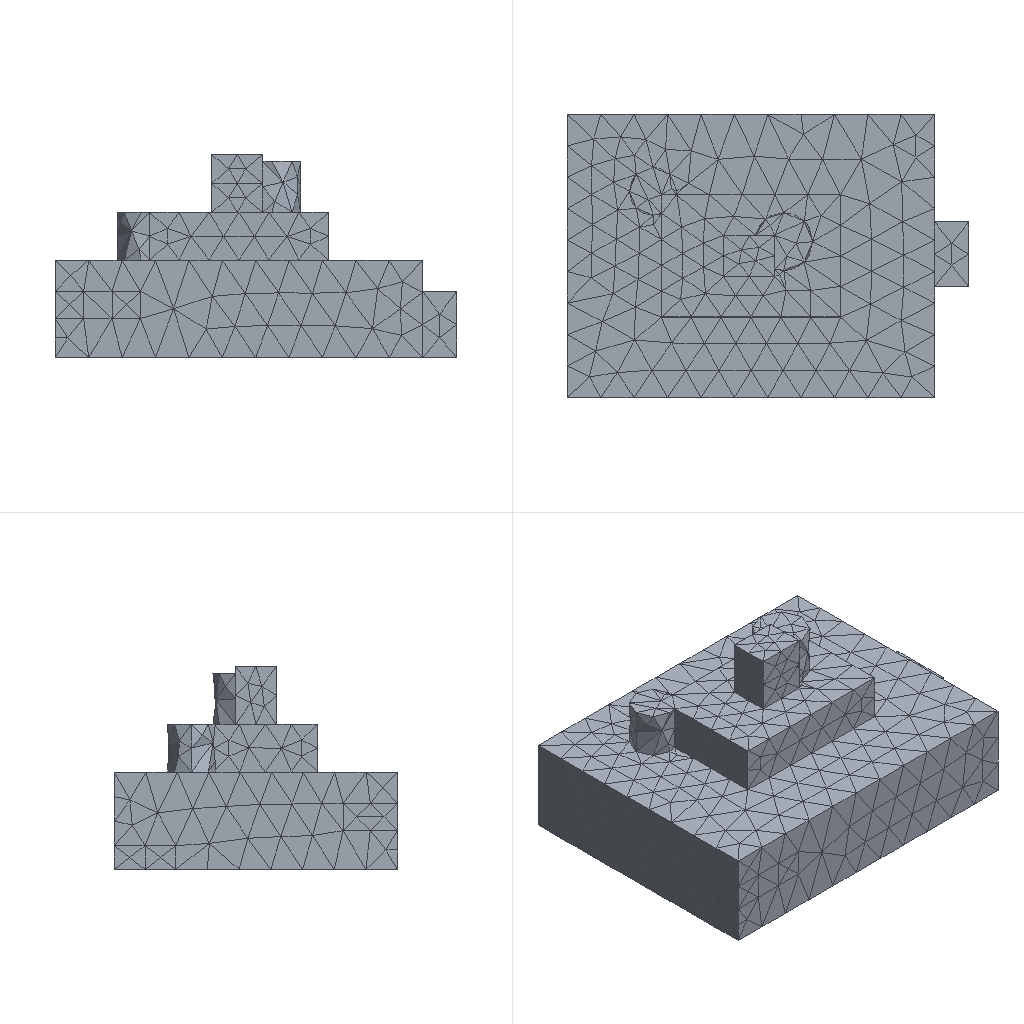Simulation study | ansys mapdl
Set-up summary:
category,name,step,type,value,unit,region
solver,ansys_mapdl
units,mm-N-s-tonne (MPa),,inferred,E=210000 density=
analysis,model,,static
mesh,nodes,,,6321
mesh,elements,,,3878
element_type,SOLID187,,,3878
material,mat 1,,E,210000
material,mat 1,,nu,0.3
load,,model,body load temp,,,all
load,,model,force,"1000 [dir=(0, 0, -1) n=330]",,node list
bc,,model,fixed,"[dofs=UX,UY,UZ n=6499]",,node list
Ansys APDL input file, long lists of numbers shortened:
/COM,ANSYS RELEASE 2026 R1           BUILD 26.1      UP20260202       09:10:15
/PREP7
/NOPR
/TITLE,2
ANTYPE, 0
*IF,_CDRDOFF,EQ,1,THEN     !if solid model was read in
_CDRDOFF=             !reset flag, numoffs already performed
*ELSE              !offset database for the following FE model
NUMOFF,NODE,     6321
NUMOFF,ELEM,     3878
NUMOFF,MAT ,        1
NUMOFF,TYPE,        1
*ENDIF
*SET,_RETURN ,  0.
*SET,_STATUS ,  0.
*SET,_UIQR   ,  330.
*SET,__FLOATPARAMETER__,  6321.
DOF,DELETE
ETBLOCK,        1,        1
(2i9,19a9)
        1      187        0        0        0        0        0        0        0        0        0        0        0        0        0        0        0        0        0        0        0
       -1
NBLOCK,6,SOLID,      6321,      6321
(3i9,6e21.13e3)
        1        0        0 7.0000000000000E+000 6.0000000000000E+000 5.9610000000000E+001
! (6320 more lines like these left out)
N,UNBL,LOC,       -1,
EBLOCK,19,SOLID,      3878,      3878
(19i10)
         1         1         1         1         0         0         0         0        10         0         1      2195      2196      2197      2198      2593      2594      2595      2596
! (7755 more lines like these left out)
        -1
MPTEMP,UNBL, 1, 1,  0.    ,
MPDATA,UNBL, 1,EX  ,       1, 1,  210000.000    ,
MPTEMP,UNBL, 1, 1,  0.    ,
MPDATA,UNBL, 1,NUXY,       1, 1, 0.3    ,
MPTEMP,UNBL, 1, 1,  0.    ,
MPDATA,UNBL, 1,PRXY,       1, 1, 0.3    ,
EXTOPT,ATTR,      0,      0,      0
EXTOPT,ESIZE,  0,  0.
EXTOPT,ACLEAR,      0
TREF,  0.
IRLF,  0
BFUNIF,TEMP,_TINY
ACEL,  0.    ,  0.    ,  0.
OMEGA,  0.    ,  0.    ,  0.
DOMEGA,  0.    ,  0.    ,  0.
CGLOC,  0.    ,  0.    ,  0.
CGOMEGA,  0.    ,  0.    ,  0.
DCGOMG,  0.    ,  0.    ,  0.
KUSE,     0
TIME,  0.
ALPHAD,  0.
BETAD,  0.
DMPRAT,  0.
DMPSTR,  0.
CRPLIM, 0.1    ,   0
CRPLIM,  0.    ,   1
NCNV,     0, 1.000000000E+12,     0,  0.    ,  0.
NEQIT,     0
ERESX,DEFA
DBLOCK,      6499
(i9,a6,2(pg16.9))
      467  UX    0.00000000      0.00000000
! (6498 more lines like these left out)
       -1
FBLOCK,       330
(i9,a6,2(pg16.9))
        1  FZ   -3.03030303      0.00000000
! (329 more lines like these left out)
       -1
/GO
FINISH
Results summary:
result,analysis_type_db,,,static,unstated
result,n_sets,,,1,unstated
result,load_steps[0].set,load_step=1,,1,unstated
result,load_steps[0].substep,load_step=1,,1,unstated
result,load_steps[0].time,load_step=1,,1,unstated
result,load_steps[0].freq,load_step=1,,1,unstated
result,load_steps[0].max_usum,load_step=1,,0.0003743,unstated
result,load_steps[0].max_seqv,load_step=1,,3.568,unstated
result,load_steps[0].reaction_sum.FX,load_step=1,,1.93108e-11,unstated
result,load_steps[0].reaction_sum.FY,load_step=1,,6.83187e-12,unstated
result,load_steps[0].reaction_sum.FZ,load_step=1,,1000,unstated
result,load_steps[0].reaction_sum.MX,load_step=1,,0,unstated
result,load_steps[0].reaction_sum.MY,load_step=1,,0,unstated
result,load_steps[0].reaction_sum.MZ,load_step=1,,0,unstated
result,convergence,,,results present for all listed sets,unstated